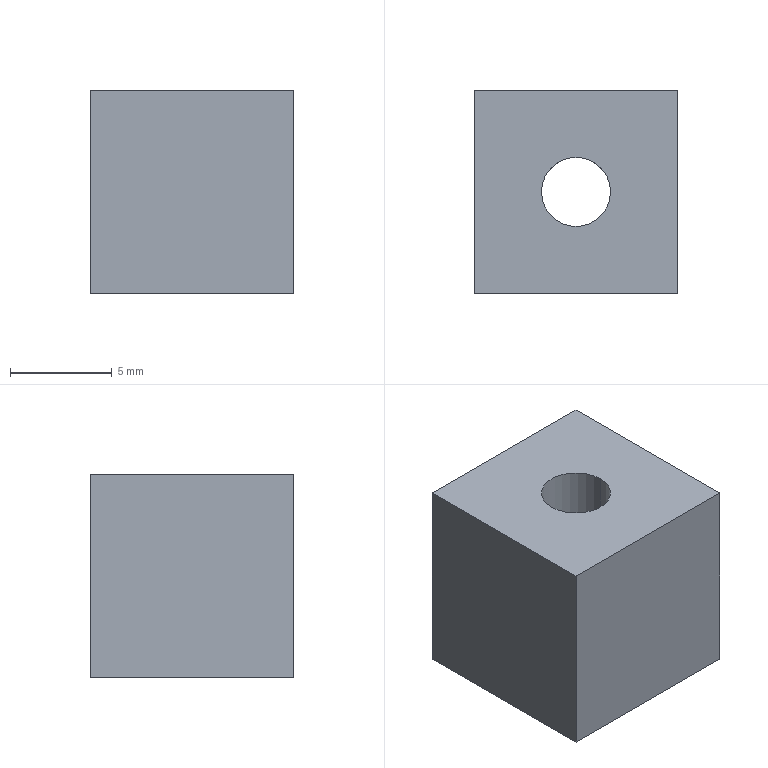Part | SolidWorks | features BaseBody 1 | 1 solid | 11 faces | box 10 x 10 x 10 mm | volume 827.255 mm3 | plane 7 | cylinder 4 | commonest cylinder face diameters 3.4 x2 6.5 x2
STEP:
#1=CARTESIAN_POINT('',(3.25,0.,3.4));
#2=VERTEX_POINT('',#1);
#3=CARTESIAN_POINT('',(-3.25,0.,3.4));
#4=VERTEX_POINT('',#3);
#5=CARTESIAN_POINT('',(0.,0.,3.4));
#6=DIRECTION('',(0.,0.,-1.));
#7=DIRECTION('',(-1.,0.,0.));
#8=AXIS2_PLACEMENT_3D('',#5,#6,#7);
#9=CIRCLE('',#8,3.25);
#10=EDGE_CURVE('',#2,#4,#9,.T.);
#11=ORIENTED_EDGE('',*,*,#10,.F.);
#12=CARTESIAN_POINT('',(3.25,0.,0.));
#13=VERTEX_POINT('',#12);
#14=CARTESIAN_POINT('',(3.25,0.,0.));
#15=DIRECTION('',(0.,0.,-1.));
#16=VECTOR('',#15,1000.);
#17=LINE('',#14,#16);
#18=EDGE_CURVE('',#2,#13,#17,.T.);
#19=ORIENTED_EDGE('',*,*,#18,.T.);
#20=CARTESIAN_POINT('',(-3.25,0.,0.));
#21=VERTEX_POINT('',#20);
#22=CARTESIAN_POINT('',(0.,0.,0.));
#23=DIRECTION('',(0.,0.,1.));
#24=DIRECTION('',(-1.,0.,0.));
#25=AXIS2_PLACEMENT_3D('',#22,#23,#24);
#26=CIRCLE('',#25,3.25);
#27=EDGE_CURVE('',#21,#13,#26,.T.);
#28=ORIENTED_EDGE('',*,*,#27,.F.);
#29=CARTESIAN_POINT('',(-3.25,0.,0.));
#30=DIRECTION('',(0.,0.,-1.));
#31=VECTOR('',#30,1000.);
#32=LINE('',#29,#31);
#33=EDGE_CURVE('',#4,#21,#32,.T.);
#34=ORIENTED_EDGE('',*,*,#33,.F.);
#35=EDGE_LOOP('',(#11,#19,#28,#34));
#36=FACE_OUTER_BOUND('',#35,.T.);
#37=CARTESIAN_POINT('',(0.,0.,0.));
#38=DIRECTION('',(0.,0.,-1.));
#39=DIRECTION('',(-1.,0.,0.));
#40=AXIS2_PLACEMENT_3D('',#37,#38,#39);
#41=CYLINDRICAL_SURFACE('',#40,3.25);
#42=ADVANCED_FACE('',(#36),#41,.F.);
#43=CARTESIAN_POINT('',(-1.7,0.,10.));
#44=VERTEX_POINT('',#43);
#45=CARTESIAN_POINT('',(1.7,0.,10.));
#46=VERTEX_POINT('',#45);
#47=CARTESIAN_POINT('',(0.,0.,10.));
#48=DIRECTION('',(0.,0.,1.));
#49=DIRECTION('',(-1.,0.,0.));
#50=AXIS2_PLACEMENT_3D('',#47,#48,#49);
#51=CIRCLE('',#50,1.7);
#52=EDGE_CURVE('',#44,#46,#51,.T.);
#53=ORIENTED_EDGE('',*,*,#52,.T.);
#54=CARTESIAN_POINT('',(1.7,0.,3.4));
#55=VERTEX_POINT('',#54);
#56=CARTESIAN_POINT('',(1.7,0.,0.));
#57=DIRECTION('',(0.,0.,-1.));
#58=VECTOR('',#57,1000.);
#59=LINE('',#56,#58);
#60=EDGE_CURVE('',#46,#55,#59,.T.);
#61=ORIENTED_EDGE('',*,*,#60,.T.);
#62=CARTESIAN_POINT('',(-1.7,0.,3.4));
#63=VERTEX_POINT('',#62);
#64=CARTESIAN_POINT('',(0.,0.,3.4));
#65=DIRECTION('',(0.,0.,1.));
#66=DIRECTION('',(-1.,0.,0.));
#67=AXIS2_PLACEMENT_3D('',#64,#65,#66);
#68=CIRCLE('',#67,1.7);
#69=EDGE_CURVE('',#63,#55,#68,.T.);
#70=ORIENTED_EDGE('',*,*,#69,.F.);
#71=CARTESIAN_POINT('',(-1.7,0.,0.));
#72=DIRECTION('',(0.,0.,-1.));
#73=VECTOR('',#72,1000.);
#74=LINE('',#71,#73);
#75=EDGE_CURVE('',#44,#63,#74,.T.);
#76=ORIENTED_EDGE('',*,*,#75,.F.);
#77=EDGE_LOOP('',(#53,#61,#70,#76));
#78=FACE_OUTER_BOUND('',#77,.T.);
#79=CARTESIAN_POINT('',(0.,0.,0.));
#80=DIRECTION('',(0.,0.,-1.));
#81=DIRECTION('',(-1.,0.,0.));
#82=AXIS2_PLACEMENT_3D('',#79,#80,#81);
#83=CYLINDRICAL_SURFACE('',#82,1.7);
#84=ADVANCED_FACE('',(#78),#83,.F.);
#85=CARTESIAN_POINT('',(5.,5.,10.));
#86=VERTEX_POINT('',#85);
#87=CARTESIAN_POINT('',(5.,5.,0.));
#88=VERTEX_POINT('',#87);
#89=CARTESIAN_POINT('',(5.,5.,10.));
#90=DIRECTION('',(0.,0.,-1.));
#91=VECTOR('',#90,1000.);
#92=LINE('',#89,#91);
#93=EDGE_CURVE('',#86,#88,#92,.T.);
#94=ORIENTED_EDGE('',*,*,#93,.F.);
#95=CARTESIAN_POINT('',(5.,-5.,10.));
#96=VERTEX_POINT('',#95);
#97=CARTESIAN_POINT('',(5.,-5.,10.));
#98=DIRECTION('',(0.,1.,0.));
#99=VECTOR('',#98,1000.);
#100=LINE('',#97,#99);
#101=EDGE_CURVE('',#96,#86,#100,.T.);
#102=ORIENTED_EDGE('',*,*,#101,.F.);
#103=CARTESIAN_POINT('',(5.,-5.,0.));
#104=VERTEX_POINT('',#103);
#105=CARTESIAN_POINT('',(5.,-5.,10.));
#106=DIRECTION('',(0.,0.,1.));
#107=VECTOR('',#106,1000.);
#108=LINE('',#105,#107);
#109=EDGE_CURVE('',#104,#96,#108,.T.);
#110=ORIENTED_EDGE('',*,*,#109,.F.);
#111=CARTESIAN_POINT('',(5.,-5.,0.));
#112=DIRECTION('',(0.,-1.,0.));
#113=VECTOR('',#112,1000.);
#114=LINE('',#111,#113);
#115=EDGE_CURVE('',#88,#104,#114,.T.);
#116=ORIENTED_EDGE('',*,*,#115,.F.);
#117=EDGE_LOOP('',(#94,#102,#110,#116));
#118=FACE_OUTER_BOUND('',#117,.T.);
#119=CARTESIAN_POINT('',(5.,-5.,10.));
#120=DIRECTION('',(-1.,0.,0.));
#121=DIRECTION('',(0.,0.,1.));
#122=AXIS2_PLACEMENT_3D('',#119,#120,#121);
#123=PLANE('',#122);
#124=ADVANCED_FACE('',(#118),#123,.F.);
#125=CARTESIAN_POINT('',(-5.,-5.,0.));
#126=VERTEX_POINT('',#125);
#127=CARTESIAN_POINT('',(-5.,5.,0.));
#128=VERTEX_POINT('',#127);
#129=CARTESIAN_POINT('',(-5.,0.,0.));
#130=DIRECTION('',(0.,1.,0.));
#131=VECTOR('',#130,1000.);
#132=LINE('',#129,#131);
#133=EDGE_CURVE('',#126,#128,#132,.T.);
#134=ORIENTED_EDGE('',*,*,#133,.T.);
#135=CARTESIAN_POINT('',(0.,5.,0.));
#136=DIRECTION('',(1.,0.,0.));
#137=VECTOR('',#136,1000.);
#138=LINE('',#135,#137);
#139=EDGE_CURVE('',#128,#88,#138,.T.);
#140=ORIENTED_EDGE('',*,*,#139,.T.);
#141=ORIENTED_EDGE('',*,*,#115,.T.);
#142=CARTESIAN_POINT('',(0.,-5.,0.));
#143=DIRECTION('',(-1.,0.,0.));
#144=VECTOR('',#143,1000.);
#145=LINE('',#142,#144);
#146=EDGE_CURVE('',#104,#126,#145,.T.);
#147=ORIENTED_EDGE('',*,*,#146,.T.);
#148=EDGE_LOOP('',(#134,#140,#141,#147));
#149=FACE_OUTER_BOUND('',#148,.T.);
#150=ORIENTED_EDGE('',*,*,#27,.T.);
#151=CARTESIAN_POINT('',(0.,0.,0.));
#152=DIRECTION('',(0.,0.,1.));
#153=DIRECTION('',(-1.,0.,0.));
#154=AXIS2_PLACEMENT_3D('',#151,#152,#153);
#155=CIRCLE('',#154,3.25);
#156=EDGE_CURVE('',#13,#21,#155,.T.);
#157=ORIENTED_EDGE('',*,*,#156,.T.);
#158=EDGE_LOOP('',(#150,#157));
#159=FACE_BOUND('',#158,.T.);
#160=CARTESIAN_POINT('',(0.,0.,0.));
#161=DIRECTION('',(0.,0.,-1.));
#162=DIRECTION('',(-1.,0.,0.));
#163=AXIS2_PLACEMENT_3D('',#160,#161,#162);
#164=PLANE('',#163);
#165=ADVANCED_FACE('',(#149,#159),#164,.T.);
#166=CARTESIAN_POINT('',(-5.,5.,10.));
#167=VERTEX_POINT('',#166);
#168=CARTESIAN_POINT('',(-5.,5.,10.));
#169=DIRECTION('',(0.,0.,-1.));
#170=VECTOR('',#169,1000.);
#171=LINE('',#168,#170);
#172=EDGE_CURVE('',#167,#128,#171,.T.);
#173=ORIENTED_EDGE('',*,*,#172,.F.);
#174=CARTESIAN_POINT('',(-5.,5.,10.));
#175=DIRECTION('',(-1.,0.,0.));
#176=VECTOR('',#175,1000.);
#177=LINE('',#174,#176);
#178=EDGE_CURVE('',#86,#167,#177,.T.);
#179=ORIENTED_EDGE('',*,*,#178,.F.);
#180=ORIENTED_EDGE('',*,*,#93,.T.);
#181=ORIENTED_EDGE('',*,*,#139,.F.);
#182=EDGE_LOOP('',(#173,#179,#180,#181));
#183=FACE_OUTER_BOUND('',#182,.T.);
#184=CARTESIAN_POINT('',(-5.,5.,10.));
#185=DIRECTION('',(0.,-1.,0.));
#186=DIRECTION('',(0.,0.,-1.));
#187=AXIS2_PLACEMENT_3D('',#184,#185,#186);
#188=PLANE('',#187);
#189=ADVANCED_FACE('',(#183),#188,.F.);
#190=ORIENTED_EDGE('',*,*,#178,.T.);
#191=CARTESIAN_POINT('',(-5.,-5.,10.));
#192=VERTEX_POINT('',#191);
#193=CARTESIAN_POINT('',(-5.,0.,10.));
#194=DIRECTION('',(0.,1.,0.));
#195=VECTOR('',#194,1000.);
#196=LINE('',#193,#195);
#197=EDGE_CURVE('',#192,#167,#196,.T.);
#198=ORIENTED_EDGE('',*,*,#197,.F.);
#199=CARTESIAN_POINT('',(0.,-5.,10.));
#200=DIRECTION('',(-1.,0.,0.));
#201=VECTOR('',#200,1000.);
#202=LINE('',#199,#201);
#203=EDGE_CURVE('',#96,#192,#202,.T.);
#204=ORIENTED_EDGE('',*,*,#203,.F.);
#205=ORIENTED_EDGE('',*,*,#101,.T.);
#206=EDGE_LOOP('',(#190,#198,#204,#205));
#207=FACE_OUTER_BOUND('',#206,.T.);
#208=ORIENTED_EDGE('',*,*,#52,.F.);
#209=CARTESIAN_POINT('',(0.,0.,10.));
#210=DIRECTION('',(0.,0.,1.));
#211=DIRECTION('',(-1.,0.,0.));
#212=AXIS2_PLACEMENT_3D('',#209,#210,#211);
#213=CIRCLE('',#212,1.7);
#214=EDGE_CURVE('',#46,#44,#213,.T.);
#215=ORIENTED_EDGE('',*,*,#214,.F.);
#216=EDGE_LOOP('',(#208,#215));
#217=FACE_BOUND('',#216,.T.);
#218=CARTESIAN_POINT('',(0.,0.,10.));
#219=DIRECTION('',(0.,0.,-1.));
#220=DIRECTION('',(-1.,0.,0.));
#221=AXIS2_PLACEMENT_3D('',#218,#219,#220);
#222=PLANE('',#221);
#223=ADVANCED_FACE('',(#207,#217),#222,.F.);
#224=ORIENTED_EDGE('',*,*,#109,.T.);
#225=ORIENTED_EDGE('',*,*,#203,.T.);
#226=CARTESIAN_POINT('',(-5.,-5.,10.));
#227=DIRECTION('',(0.,0.,1.));
#228=VECTOR('',#227,1000.);
#229=LINE('',#226,#228);
#230=EDGE_CURVE('',#126,#192,#229,.T.);
#231=ORIENTED_EDGE('',*,*,#230,.F.);
#232=ORIENTED_EDGE('',*,*,#146,.F.);
#233=EDGE_LOOP('',(#224,#225,#231,#232));
#234=FACE_OUTER_BOUND('',#233,.T.);
#235=CARTESIAN_POINT('',(-5.,-5.,10.));
#236=DIRECTION('',(0.,1.,0.));
#237=DIRECTION('',(0.,0.,1.));
#238=AXIS2_PLACEMENT_3D('',#235,#236,#237);
#239=PLANE('',#238);
#240=ADVANCED_FACE('',(#234),#239,.F.);
#241=ORIENTED_EDGE('',*,*,#230,.T.);
#242=ORIENTED_EDGE('',*,*,#197,.T.);
#243=ORIENTED_EDGE('',*,*,#172,.T.);
#244=ORIENTED_EDGE('',*,*,#133,.F.);
#245=EDGE_LOOP('',(#241,#242,#243,#244));
#246=FACE_OUTER_BOUND('',#245,.T.);
#247=CARTESIAN_POINT('',(-5.,-5.,10.));
#248=DIRECTION('',(1.,0.,0.));
#249=DIRECTION('',(0.,0.,-1.));
#250=AXIS2_PLACEMENT_3D('',#247,#248,#249);
#251=PLANE('',#250);
#252=ADVANCED_FACE('',(#246),#251,.F.);
#253=ORIENTED_EDGE('',*,*,#18,.F.);
#254=CARTESIAN_POINT('',(0.,0.,3.4));
#255=DIRECTION('',(0.,0.,-1.));
#256=DIRECTION('',(-1.,0.,0.));
#257=AXIS2_PLACEMENT_3D('',#254,#255,#256);
#258=CIRCLE('',#257,3.25);
#259=EDGE_CURVE('',#4,#2,#258,.T.);
#260=ORIENTED_EDGE('',*,*,#259,.F.);
#261=ORIENTED_EDGE('',*,*,#33,.T.);
#262=ORIENTED_EDGE('',*,*,#156,.F.);
#263=EDGE_LOOP('',(#253,#260,#261,#262));
#264=FACE_OUTER_BOUND('',#263,.T.);
#265=CARTESIAN_POINT('',(0.,0.,0.));
#266=DIRECTION('',(0.,0.,-1.));
#267=DIRECTION('',(-1.,0.,0.));
#268=AXIS2_PLACEMENT_3D('',#265,#266,#267);
#269=CYLINDRICAL_SURFACE('',#268,3.25);
#270=ADVANCED_FACE('',(#264),#269,.F.);
#271=ORIENTED_EDGE('',*,*,#60,.F.);
#272=ORIENTED_EDGE('',*,*,#214,.T.);
#273=ORIENTED_EDGE('',*,*,#75,.T.);
#274=CARTESIAN_POINT('',(0.,0.,3.4));
#275=DIRECTION('',(0.,0.,1.));
#276=DIRECTION('',(-1.,0.,0.));
#277=AXIS2_PLACEMENT_3D('',#274,#275,#276);
#278=CIRCLE('',#277,1.7);
#279=EDGE_CURVE('',#55,#63,#278,.T.);
#280=ORIENTED_EDGE('',*,*,#279,.F.);
#281=EDGE_LOOP('',(#271,#272,#273,#280));
#282=FACE_OUTER_BOUND('',#281,.T.);
#283=CARTESIAN_POINT('',(0.,0.,0.));
#284=DIRECTION('',(0.,0.,-1.));
#285=DIRECTION('',(-1.,0.,0.));
#286=AXIS2_PLACEMENT_3D('',#283,#284,#285);
#287=CYLINDRICAL_SURFACE('',#286,1.7);
#288=ADVANCED_FACE('',(#282),#287,.F.);
#289=ORIENTED_EDGE('',*,*,#259,.T.);
#290=ORIENTED_EDGE('',*,*,#10,.T.);
#291=EDGE_LOOP('',(#289,#290));
#292=FACE_OUTER_BOUND('',#291,.T.);
#293=ORIENTED_EDGE('',*,*,#69,.T.);
#294=ORIENTED_EDGE('',*,*,#279,.T.);
#295=EDGE_LOOP('',(#293,#294));
#296=FACE_BOUND('',#295,.T.);
#297=CARTESIAN_POINT('',(1.7,0.,3.4));
#298=DIRECTION('',(0.,0.,1.));
#299=DIRECTION('',(1.,0.,0.));
#300=AXIS2_PLACEMENT_3D('',#297,#298,#299);
#301=PLANE('',#300);
#302=ADVANCED_FACE('',(#292,#296),#301,.F.);
#303=CLOSED_SHELL('',(#42,#84,#124,#165,#189,#223,#240,#252,#270,#288,#302));
#304=MANIFOLD_SOLID_BREP('',#303);
#305=CARTESIAN_POINT('',(0.,0.,0.));
#306=DIRECTION('',(0.,0.,1.));
#307=DIRECTION('',(1.,0.,0.));
#308=AXIS2_PLACEMENT_3D('',#305,#306,#307);
#309=(LENGTH_UNIT()NAMED_UNIT(*)SI_UNIT(.MILLI.,.METRE.));
#310=UNCERTAINTY_MEASURE_WITH_UNIT(LENGTH_MEASURE(0.00001),#309,'','');
#311=(NAMED_UNIT(*)PLANE_ANGLE_UNIT()SI_UNIT($,.RADIAN.));
#312=(NAMED_UNIT(*)SI_UNIT($,.STERADIAN.)SOLID_ANGLE_UNIT());
#313=(GEOMETRIC_REPRESENTATION_CONTEXT(3)GLOBAL_UNCERTAINTY_ASSIGNED_CONTEXT((#310))GLOBAL_UNIT_ASSIGNED_CONTEXT((#309,#311,#312))REPRESENTATION_CONTEXT('',''));
#314=ADVANCED_BREP_SHAPE_REPRESENTATION('',(#304,#308),#313);